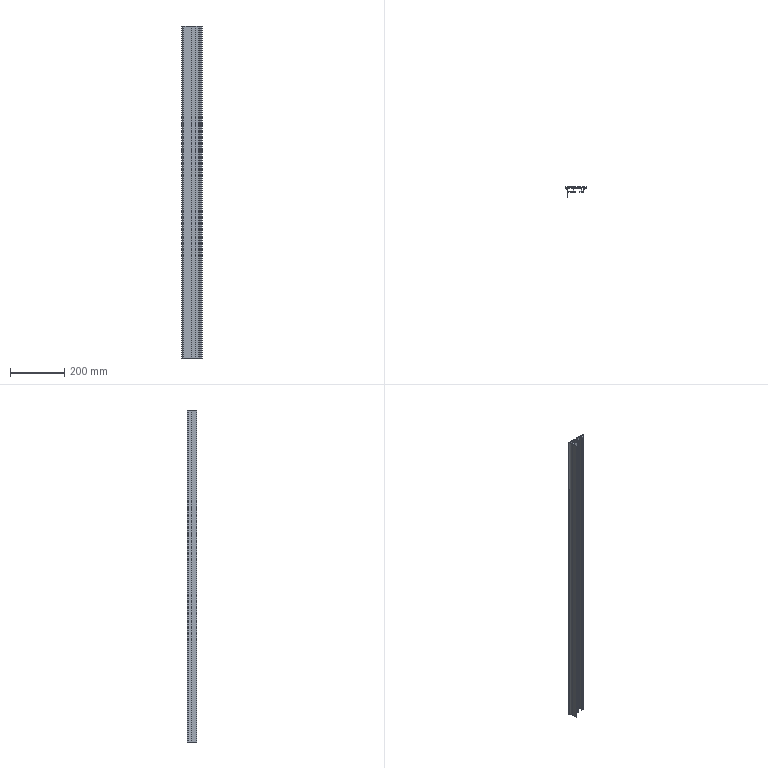Part | STEP file | SIDE | 1 solid | 100 faces | box 76 x 36.5 x 1228 mm | volume 489204 mm3 | plane 72 | cylinder 28 | commonest cylinder face diameters 1 x17 3.625 x4 6 x3 2 x2 40 x1 44 x1